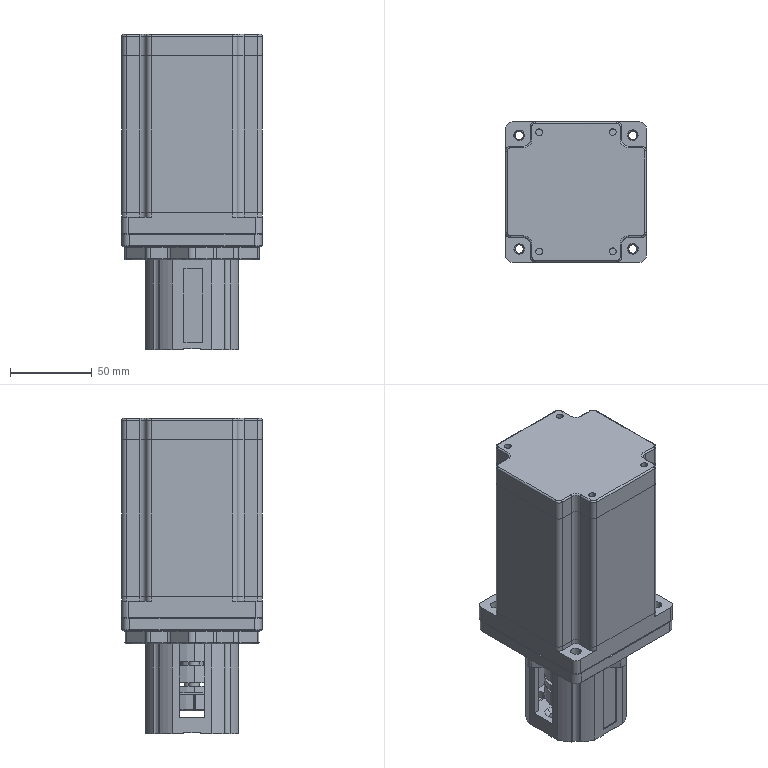Part | STEP file | Copy of 86 motor assembly (universal motor base)^K50A-1H20-S(formula driven)-L300-motor left- | 7 solids | 676 faces | box 86.045 x 86.045 x 193 mm | volume 941997 mm3 | cylinder 359 | plane 181 | cone 76 | torus 60 | commonest cylinder face diameters 8 x52 6 x51 1 x40 7 x28 4.2 x24 2 x18